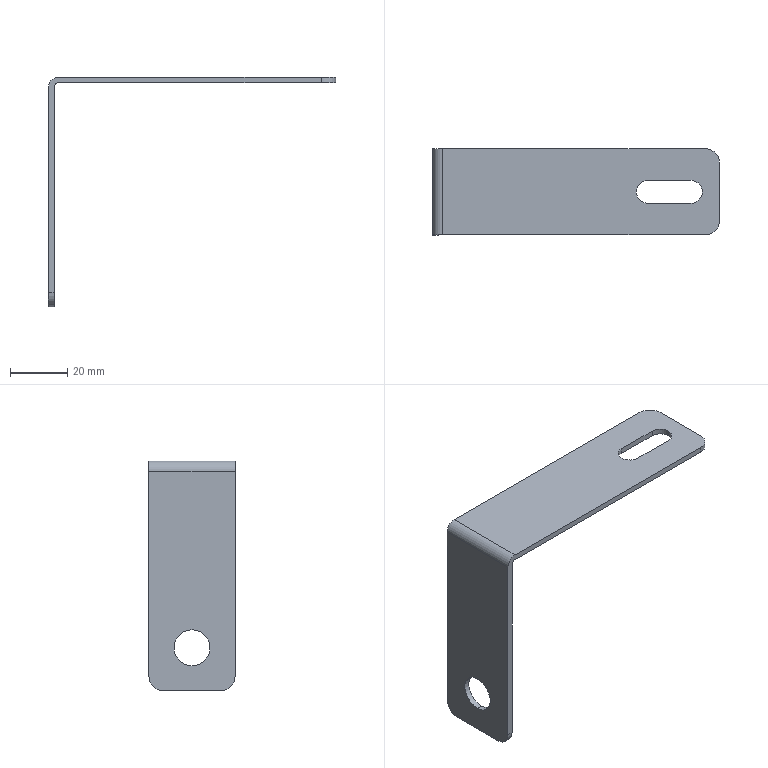Part | SolidWorks | features BaseBody 1 | 1 solid | 21 faces | box 100 x 30 x 80 mm | volume 9987 mm3 | cylinder 11 | plane 10 | commonest cylinder face diameters 10 x4 8 x3 12.5 x2 3 x1 7 x1
STEP:
#1=CARTESIAN_POINT('',(44.,0.,-2.));
#2=VERTEX_POINT('',#1);
#3=CARTESIAN_POINT('',(40.,4.,-2.));
#4=VERTEX_POINT('',#3);
#5=CARTESIAN_POINT('',(40.,0.,-2.));
#6=DIRECTION('',(0.,0.,1.));
#7=DIRECTION('',(1.,0.,0.));
#8=AXIS2_PLACEMENT_3D('',#5,#6,#7);
#9=CIRCLE('',#8,4.);
#10=EDGE_CURVE('',#2,#4,#9,.T.);
#11=ORIENTED_EDGE('',*,*,#10,.F.);
#12=CARTESIAN_POINT('',(44.,0.,0.));
#13=VERTEX_POINT('',#12);
#14=CARTESIAN_POINT('',(44.,0.,-10.));
#15=DIRECTION('',(0.,0.,1.));
#16=VECTOR('',#15,1000.);
#17=LINE('',#14,#16);
#18=EDGE_CURVE('',#2,#13,#17,.T.);
#19=ORIENTED_EDGE('',*,*,#18,.T.);
#20=CARTESIAN_POINT('',(40.,4.,0.));
#21=VERTEX_POINT('',#20);
#22=CARTESIAN_POINT('',(40.,0.,0.));
#23=DIRECTION('',(0.,0.,1.));
#24=DIRECTION('',(1.,0.,0.));
#25=AXIS2_PLACEMENT_3D('',#22,#23,#24);
#26=CIRCLE('',#25,4.);
#27=EDGE_CURVE('',#13,#21,#26,.T.);
#28=ORIENTED_EDGE('',*,*,#27,.T.);
#29=CARTESIAN_POINT('',(40.,4.,-10.));
#30=DIRECTION('',(0.,0.,-1.));
#31=VECTOR('',#30,1000.);
#32=LINE('',#29,#31);
#33=EDGE_CURVE('',#21,#4,#32,.T.);
#34=ORIENTED_EDGE('',*,*,#33,.T.);
#35=EDGE_LOOP('',(#11,#19,#28,#34));
#36=FACE_OUTER_BOUND('',#35,.T.);
#37=CARTESIAN_POINT('',(40.,0.,-10.));
#38=DIRECTION('',(0.,0.,1.));
#39=DIRECTION('',(1.,0.,0.));
#40=AXIS2_PLACEMENT_3D('',#37,#38,#39);
#41=CYLINDRICAL_SURFACE('',#40,4.);
#42=ADVANCED_FACE('',(#36),#41,.F.);
#43=CARTESIAN_POINT('',(-48.,0.,-71.25));
#44=VERTEX_POINT('',#43);
#45=CARTESIAN_POINT('',(-48.,0.,-58.75));
#46=VERTEX_POINT('',#45);
#47=CARTESIAN_POINT('',(-48.,0.,-65.));
#48=DIRECTION('',(-1.,0.,0.));
#49=DIRECTION('',(0.,0.,1.));
#50=AXIS2_PLACEMENT_3D('',#47,#48,#49);
#51=CIRCLE('',#50,6.25);
#52=EDGE_CURVE('',#44,#46,#51,.T.);
#53=ORIENTED_EDGE('',*,*,#52,.F.);
#54=CARTESIAN_POINT('',(-50.,0.,-71.25));
#55=VERTEX_POINT('',#54);
#56=CARTESIAN_POINT('',(-40.,0.,-71.25));
#57=DIRECTION('',(-1.,0.,0.));
#58=VECTOR('',#57,1000.);
#59=LINE('',#56,#58);
#60=EDGE_CURVE('',#44,#55,#59,.T.);
#61=ORIENTED_EDGE('',*,*,#60,.T.);
#62=CARTESIAN_POINT('',(-50.,0.,-58.75));
#63=VERTEX_POINT('',#62);
#64=CARTESIAN_POINT('',(-50.,0.,-65.));
#65=DIRECTION('',(1.,0.,0.));
#66=DIRECTION('',(0.,0.,1.));
#67=AXIS2_PLACEMENT_3D('',#64,#65,#66);
#68=CIRCLE('',#67,6.25);
#69=EDGE_CURVE('',#63,#55,#68,.T.);
#70=ORIENTED_EDGE('',*,*,#69,.F.);
#71=CARTESIAN_POINT('',(-40.,0.,-58.75));
#72=DIRECTION('',(-1.,0.,0.));
#73=VECTOR('',#72,1000.);
#74=LINE('',#71,#73);
#75=EDGE_CURVE('',#46,#63,#74,.T.);
#76=ORIENTED_EDGE('',*,*,#75,.F.);
#77=EDGE_LOOP('',(#53,#61,#70,#76));
#78=FACE_OUTER_BOUND('',#77,.T.);
#79=CARTESIAN_POINT('',(-40.,0.,-65.));
#80=DIRECTION('',(-1.,0.,0.));
#81=DIRECTION('',(0.,0.,1.));
#82=AXIS2_PLACEMENT_3D('',#79,#80,#81);
#83=CYLINDRICAL_SURFACE('',#82,6.25);
#84=ADVANCED_FACE('',(#78),#83,.F.);
#85=CARTESIAN_POINT('',(45.,15.,0.));
#86=VERTEX_POINT('',#85);
#87=CARTESIAN_POINT('',(50.,10.,0.));
#88=VERTEX_POINT('',#87);
#89=CARTESIAN_POINT('',(45.,10.,0.));
#90=DIRECTION('',(0.,0.,-1.));
#91=DIRECTION('',(1.,0.,0.));
#92=AXIS2_PLACEMENT_3D('',#89,#90,#91);
#93=CIRCLE('',#92,5.);
#94=EDGE_CURVE('',#86,#88,#93,.T.);
#95=ORIENTED_EDGE('',*,*,#94,.F.);
#96=CARTESIAN_POINT('',(-46.5,15.,0.));
#97=VERTEX_POINT('',#96);
#98=CARTESIAN_POINT('',(0.,15.,0.));
#99=DIRECTION('',(1.,0.,0.));
#100=VECTOR('',#99,1000.);
#101=LINE('',#98,#100);
#102=EDGE_CURVE('',#97,#86,#101,.T.);
#103=ORIENTED_EDGE('',*,*,#102,.F.);
#104=CARTESIAN_POINT('',(-46.5,-15.,0.));
#105=VERTEX_POINT('',#104);
#106=CARTESIAN_POINT('',(-46.5,0.,0.));
#107=DIRECTION('',(0.,1.,0.));
#108=VECTOR('',#107,1000.);
#109=LINE('',#106,#108);
#110=EDGE_CURVE('',#105,#97,#109,.T.);
#111=ORIENTED_EDGE('',*,*,#110,.F.);
#112=CARTESIAN_POINT('',(45.,-15.,0.));
#113=VERTEX_POINT('',#112);
#114=CARTESIAN_POINT('',(0.,-15.,0.));
#115=DIRECTION('',(-1.,0.,0.));
#116=VECTOR('',#115,1000.);
#117=LINE('',#114,#116);
#118=EDGE_CURVE('',#113,#105,#117,.T.);
#119=ORIENTED_EDGE('',*,*,#118,.F.);
#120=CARTESIAN_POINT('',(50.,-10.,0.));
#121=VERTEX_POINT('',#120);
#122=CARTESIAN_POINT('',(45.,-10.,0.));
#123=DIRECTION('',(0.,0.,-1.));
#124=DIRECTION('',(1.,0.,0.));
#125=AXIS2_PLACEMENT_3D('',#122,#123,#124);
#126=CIRCLE('',#125,5.);
#127=EDGE_CURVE('',#121,#113,#126,.T.);
#128=ORIENTED_EDGE('',*,*,#127,.F.);
#129=CARTESIAN_POINT('',(50.,0.,0.));
#130=DIRECTION('',(0.,-1.,0.));
#131=VECTOR('',#130,1000.);
#132=LINE('',#129,#131);
#133=EDGE_CURVE('',#88,#121,#132,.T.);
#134=ORIENTED_EDGE('',*,*,#133,.F.);
#135=EDGE_LOOP('',(#95,#103,#111,#119,#128,#134));
#136=FACE_OUTER_BOUND('',#135,.T.);
#137=CARTESIAN_POINT('',(25.,4.,0.));
#138=VERTEX_POINT('',#137);
#139=CARTESIAN_POINT('',(25.,-4.,0.));
#140=VERTEX_POINT('',#139);
#141=CARTESIAN_POINT('',(25.,0.,0.));
#142=DIRECTION('',(0.,0.,1.));
#143=DIRECTION('',(1.,0.,0.));
#144=AXIS2_PLACEMENT_3D('',#141,#142,#143);
#145=CIRCLE('',#144,4.);
#146=EDGE_CURVE('',#138,#140,#145,.T.);
#147=ORIENTED_EDGE('',*,*,#146,.F.);
#148=CARTESIAN_POINT('',(0.,4.,0.));
#149=DIRECTION('',(-1.,0.,0.));
#150=VECTOR('',#149,1000.);
#151=LINE('',#148,#150);
#152=EDGE_CURVE('',#21,#138,#151,.T.);
#153=ORIENTED_EDGE('',*,*,#152,.F.);
#154=ORIENTED_EDGE('',*,*,#27,.F.);
#155=CARTESIAN_POINT('',(40.,-4.,0.));
#156=VERTEX_POINT('',#155);
#157=CARTESIAN_POINT('',(40.,0.,0.));
#158=DIRECTION('',(0.,0.,1.));
#159=DIRECTION('',(1.,0.,0.));
#160=AXIS2_PLACEMENT_3D('',#157,#158,#159);
#161=CIRCLE('',#160,4.);
#162=EDGE_CURVE('',#156,#13,#161,.T.);
#163=ORIENTED_EDGE('',*,*,#162,.F.);
#164=CARTESIAN_POINT('',(0.,-4.,0.));
#165=DIRECTION('',(1.,0.,0.));
#166=VECTOR('',#165,1000.);
#167=LINE('',#164,#166);
#168=EDGE_CURVE('',#140,#156,#167,.T.);
#169=ORIENTED_EDGE('',*,*,#168,.F.);
#170=EDGE_LOOP('',(#147,#153,#154,#163,#169));
#171=FACE_BOUND('',#170,.T.);
#172=CARTESIAN_POINT('',(0.,0.,0.));
#173=DIRECTION('',(0.,0.,-1.));
#174=DIRECTION('',(-1.,0.,0.));
#175=AXIS2_PLACEMENT_3D('',#172,#173,#174);
#176=PLANE('',#175);
#177=ADVANCED_FACE('',(#136,#171),#176,.F.);
#178=ORIENTED_EDGE('',*,*,#133,.T.);
#179=CARTESIAN_POINT('',(50.,-10.,-2.));
#180=VERTEX_POINT('',#179);
#181=CARTESIAN_POINT('',(50.,-10.,-2.));
#182=DIRECTION('',(0.,0.,-1.));
#183=VECTOR('',#182,1000.);
#184=LINE('',#181,#183);
#185=EDGE_CURVE('',#121,#180,#184,.T.);
#186=ORIENTED_EDGE('',*,*,#185,.T.);
#187=CARTESIAN_POINT('',(50.,10.,-2.));
#188=VERTEX_POINT('',#187);
#189=CARTESIAN_POINT('',(50.,-15.,-2.));
#190=DIRECTION('',(0.,1.,0.));
#191=VECTOR('',#190,1000.);
#192=LINE('',#189,#191);
#193=EDGE_CURVE('',#180,#188,#192,.T.);
#194=ORIENTED_EDGE('',*,*,#193,.T.);
#195=CARTESIAN_POINT('',(50.,10.,-2.));
#196=DIRECTION('',(0.,0.,1.));
#197=VECTOR('',#196,1000.);
#198=LINE('',#195,#197);
#199=EDGE_CURVE('',#188,#88,#198,.T.);
#200=ORIENTED_EDGE('',*,*,#199,.T.);
#201=EDGE_LOOP('',(#178,#186,#194,#200));
#202=FACE_OUTER_BOUND('',#201,.T.);
#203=CARTESIAN_POINT('',(50.,-15.,-2.));
#204=DIRECTION('',(1.,0.,0.));
#205=DIRECTION('',(0.,0.,-1.));
#206=AXIS2_PLACEMENT_3D('',#203,#204,#205);
#207=PLANE('',#206);
#208=ADVANCED_FACE('',(#202),#207,.T.);
#209=ORIENTED_EDGE('',*,*,#94,.T.);
#210=ORIENTED_EDGE('',*,*,#199,.F.);
#211=CARTESIAN_POINT('',(45.,15.,-2.));
#212=VERTEX_POINT('',#211);
#213=CARTESIAN_POINT('',(45.,10.,-2.));
#214=DIRECTION('',(0.,0.,1.));
#215=DIRECTION('',(1.,0.,0.));
#216=AXIS2_PLACEMENT_3D('',#213,#214,#215);
#217=CIRCLE('',#216,5.);
#218=EDGE_CURVE('',#188,#212,#217,.T.);
#219=ORIENTED_EDGE('',*,*,#218,.T.);
#220=CARTESIAN_POINT('',(45.,15.,-2.));
#221=DIRECTION('',(0.,0.,1.));
#222=VECTOR('',#221,1000.);
#223=LINE('',#220,#222);
#224=EDGE_CURVE('',#212,#86,#223,.T.);
#225=ORIENTED_EDGE('',*,*,#224,.T.);
#226=EDGE_LOOP('',(#209,#210,#219,#225));
#227=FACE_OUTER_BOUND('',#226,.T.);
#228=CARTESIAN_POINT('',(45.,10.,-2.));
#229=DIRECTION('',(0.,0.,1.));
#230=DIRECTION('',(1.,0.,0.));
#231=AXIS2_PLACEMENT_3D('',#228,#229,#230);
#232=CYLINDRICAL_SURFACE('',#231,5.);
#233=ADVANCED_FACE('',(#227),#232,.T.);
#234=CARTESIAN_POINT('',(-46.5,15.,-2.));
#235=VERTEX_POINT('',#234);
#236=CARTESIAN_POINT('',(-50.,15.,-2.));
#237=DIRECTION('',(-1.,0.,0.));
#238=VECTOR('',#237,1000.);
#239=LINE('',#236,#238);
#240=EDGE_CURVE('',#212,#235,#239,.T.);
#241=ORIENTED_EDGE('',*,*,#240,.T.);
#242=CARTESIAN_POINT('',(-48.,15.,-3.5));
#243=VERTEX_POINT('',#242);
#244=CARTESIAN_POINT('',(-46.5,15.,-3.5));
#245=DIRECTION('',(0.,1.,0.));
#246=DIRECTION('',(0.,0.,1.));
#247=AXIS2_PLACEMENT_3D('',#244,#245,#246);
#248=CIRCLE('',#247,1.5);
#249=EDGE_CURVE('',#243,#235,#248,.T.);
#250=ORIENTED_EDGE('',*,*,#249,.F.);
#251=CARTESIAN_POINT('',(-48.,15.,-75.));
#252=VERTEX_POINT('',#251);
#253=CARTESIAN_POINT('',(-48.,15.,-2.));
#254=DIRECTION('',(0.,0.,-1.));
#255=VECTOR('',#254,1000.);
#256=LINE('',#253,#255);
#257=EDGE_CURVE('',#243,#252,#256,.T.);
#258=ORIENTED_EDGE('',*,*,#257,.T.);
#259=CARTESIAN_POINT('',(-50.,15.,-75.));
#260=VERTEX_POINT('',#259);
#261=CARTESIAN_POINT('',(-50.,15.,-75.));
#262=DIRECTION('',(-1.,0.,0.));
#263=VECTOR('',#262,1000.);
#264=LINE('',#261,#263);
#265=EDGE_CURVE('',#252,#260,#264,.T.);
#266=ORIENTED_EDGE('',*,*,#265,.T.);
#267=CARTESIAN_POINT('',(-50.,15.,-3.5));
#268=VERTEX_POINT('',#267);
#269=CARTESIAN_POINT('',(-50.,15.,0.));
#270=DIRECTION('',(0.,0.,-1.));
#271=VECTOR('',#270,1000.);
#272=LINE('',#269,#271);
#273=EDGE_CURVE('',#268,#260,#272,.T.);
#274=ORIENTED_EDGE('',*,*,#273,.F.);
#275=CARTESIAN_POINT('',(-46.5,15.,-3.5));
#276=DIRECTION('',(0.,-1.,0.));
#277=DIRECTION('',(0.,0.,1.));
#278=AXIS2_PLACEMENT_3D('',#275,#276,#277);
#279=CIRCLE('',#278,3.5);
#280=EDGE_CURVE('',#97,#268,#279,.T.);
#281=ORIENTED_EDGE('',*,*,#280,.F.);
#282=ORIENTED_EDGE('',*,*,#102,.T.);
#283=ORIENTED_EDGE('',*,*,#224,.F.);
#284=EDGE_LOOP('',(#241,#250,#258,#266,#274,#281,#282,#283));
#285=FACE_OUTER_BOUND('',#284,.T.);
#286=CARTESIAN_POINT('',(-50.,15.,-2.));
#287=DIRECTION('',(0.,1.,0.));
#288=DIRECTION('',(0.,0.,1.));
#289=AXIS2_PLACEMENT_3D('',#286,#287,#288);
#290=PLANE('',#289);
#291=ADVANCED_FACE('',(#285),#290,.T.);
#292=CARTESIAN_POINT('',(-50.,-15.,-3.5));
#293=VERTEX_POINT('',#292);
#294=CARTESIAN_POINT('',(-50.,15.,-3.5));
#295=DIRECTION('',(0.,-1.,0.));
#296=VECTOR('',#295,1000.);
#297=LINE('',#294,#296);
#298=EDGE_CURVE('',#268,#293,#297,.T.);
#299=ORIENTED_EDGE('',*,*,#298,.T.);
#300=CARTESIAN_POINT('',(-46.5,-15.,-3.5));
#301=DIRECTION('',(0.,1.,0.));
#302=DIRECTION('',(0.,0.,1.));
#303=AXIS2_PLACEMENT_3D('',#300,#301,#302);
#304=CIRCLE('',#303,3.5);
#305=EDGE_CURVE('',#293,#105,#304,.T.);
#306=ORIENTED_EDGE('',*,*,#305,.T.);
#307=ORIENTED_EDGE('',*,*,#110,.T.);
#308=ORIENTED_EDGE('',*,*,#280,.T.);
#309=EDGE_LOOP('',(#299,#306,#307,#308));
#310=FACE_OUTER_BOUND('',#309,.T.);
#311=CARTESIAN_POINT('',(-46.5,15.,-3.5));
#312=DIRECTION('',(0.,1.,0.));
#313=DIRECTION('',(0.,0.,1.));
#314=AXIS2_PLACEMENT_3D('',#311,#312,#313);
#315=CYLINDRICAL_SURFACE('',#314,3.5);
#316=ADVANCED_FACE('',(#310),#315,.T.);
#317=ORIENTED_EDGE('',*,*,#118,.T.);
#318=ORIENTED_EDGE('',*,*,#305,.F.);
#319=CARTESIAN_POINT('',(-50.,-15.,-75.));
#320=VERTEX_POINT('',#319);
#321=CARTESIAN_POINT('',(-50.,-15.,0.));
#322=DIRECTION('',(0.,0.,1.));
#323=VECTOR('',#322,1000.);
#324=LINE('',#321,#323);
#325=EDGE_CURVE('',#320,#293,#324,.T.);
#326=ORIENTED_EDGE('',*,*,#325,.F.);
#327=CARTESIAN_POINT('',(-48.,-15.,-75.));
#328=VERTEX_POINT('',#327);
#329=CARTESIAN_POINT('',(-50.,-15.,-75.));
#330=DIRECTION('',(1.,0.,0.));
#331=VECTOR('',#330,1000.);
#332=LINE('',#329,#331);
#333=EDGE_CURVE('',#320,#328,#332,.T.);
#334=ORIENTED_EDGE('',*,*,#333,.T.);
#335=CARTESIAN_POINT('',(-48.,-15.,-3.5));
#336=VERTEX_POINT('',#335);
#337=CARTESIAN_POINT('',(-48.,-15.,-80.));
#338=DIRECTION('',(0.,0.,1.));
#339=VECTOR('',#338,1000.);
#340=LINE('',#337,#339);
#341=EDGE_CURVE('',#328,#336,#340,.T.);
#342=ORIENTED_EDGE('',*,*,#341,.T.);
#343=CARTESIAN_POINT('',(-46.5,-15.,-2.));
#344=VERTEX_POINT('',#343);
#345=CARTESIAN_POINT('',(-46.5,-15.,-3.5));
#346=DIRECTION('',(0.,1.,0.));
#347=DIRECTION('',(0.,0.,1.));
#348=AXIS2_PLACEMENT_3D('',#345,#346,#347);
#349=CIRCLE('',#348,1.5);
#350=EDGE_CURVE('',#336,#344,#349,.T.);
#351=ORIENTED_EDGE('',*,*,#350,.T.);
#352=CARTESIAN_POINT('',(45.,-15.,-2.));
#353=VERTEX_POINT('',#352);
#354=CARTESIAN_POINT('',(-50.,-15.,-2.));
#355=DIRECTION('',(1.,0.,0.));
#356=VECTOR('',#355,1000.);
#357=LINE('',#354,#356);
#358=EDGE_CURVE('',#344,#353,#357,.T.);
#359=ORIENTED_EDGE('',*,*,#358,.T.);
#360=CARTESIAN_POINT('',(45.,-15.,-2.));
#361=DIRECTION('',(0.,0.,1.));
#362=VECTOR('',#361,1000.);
#363=LINE('',#360,#362);
#364=EDGE_CURVE('',#353,#113,#363,.T.);
#365=ORIENTED_EDGE('',*,*,#364,.T.);
#366=EDGE_LOOP('',(#317,#318,#326,#334,#342,#351,#359,#365));
#367=FACE_OUTER_BOUND('',#366,.T.);
#368=CARTESIAN_POINT('',(-50.,-15.,-2.));
#369=DIRECTION('',(0.,-1.,0.));
#370=DIRECTION('',(0.,0.,-1.));
#371=AXIS2_PLACEMENT_3D('',#368,#369,#370);
#372=PLANE('',#371);
#373=ADVANCED_FACE('',(#367),#372,.T.);
#374=ORIENTED_EDGE('',*,*,#127,.T.);
#375=ORIENTED_EDGE('',*,*,#364,.F.);
#376=CARTESIAN_POINT('',(45.,-10.,-2.));
#377=DIRECTION('',(0.,0.,1.));
#378=DIRECTION('',(1.,0.,0.));
#379=AXIS2_PLACEMENT_3D('',#376,#377,#378);
#380=CIRCLE('',#379,5.);
#381=EDGE_CURVE('',#353,#180,#380,.T.);
#382=ORIENTED_EDGE('',*,*,#381,.T.);
#383=ORIENTED_EDGE('',*,*,#185,.F.);
#384=EDGE_LOOP('',(#374,#375,#382,#383));
#385=FACE_OUTER_BOUND('',#384,.T.);
#386=CARTESIAN_POINT('',(45.,-10.,-2.));
#387=DIRECTION('',(0.,0.,1.));
#388=DIRECTION('',(1.,0.,0.));
#389=AXIS2_PLACEMENT_3D('',#386,#387,#388);
#390=CYLINDRICAL_SURFACE('',#389,5.);
#391=ADVANCED_FACE('',(#385),#390,.T.);
#392=CARTESIAN_POINT('',(25.,-4.,-2.));
#393=VERTEX_POINT('',#392);
#394=CARTESIAN_POINT('',(25.,-4.,-10.));
#395=DIRECTION('',(0.,0.,-1.));
#396=VECTOR('',#395,1000.);
#397=LINE('',#394,#396);
#398=EDGE_CURVE('',#140,#393,#397,.T.);
#399=ORIENTED_EDGE('',*,*,#398,.F.);
#400=ORIENTED_EDGE('',*,*,#168,.T.);
#401=CARTESIAN_POINT('',(40.,-4.,-2.));
#402=VERTEX_POINT('',#401);
#403=CARTESIAN_POINT('',(40.,-4.,-10.));
#404=DIRECTION('',(0.,0.,1.));
#405=VECTOR('',#404,1000.);
#406=LINE('',#403,#405);
#407=EDGE_CURVE('',#402,#156,#406,.T.);
#408=ORIENTED_EDGE('',*,*,#407,.F.);
#409=CARTESIAN_POINT('',(25.,-4.,-2.));
#410=DIRECTION('',(1.,0.,0.));
#411=VECTOR('',#410,1000.);
#412=LINE('',#409,#411);
#413=EDGE_CURVE('',#393,#402,#412,.T.);
#414=ORIENTED_EDGE('',*,*,#413,.F.);
#415=EDGE_LOOP('',(#399,#400,#408,#414));
#416=FACE_OUTER_BOUND('',#415,.T.);
#417=CARTESIAN_POINT('',(25.,-4.,-10.));
#418=DIRECTION('',(0.,-1.,0.));
#419=DIRECTION('',(0.,0.,-1.));
#420=AXIS2_PLACEMENT_3D('',#417,#418,#419);
#421=PLANE('',#420);
#422=ADVANCED_FACE('',(#416),#421,.F.);
#423=CARTESIAN_POINT('',(25.,4.,-2.));
#424=VERTEX_POINT('',#423);
#425=CARTESIAN_POINT('',(25.,4.,-10.));
#426=DIRECTION('',(0.,0.,-1.));
#427=VECTOR('',#426,1000.);
#428=LINE('',#425,#427);
#429=EDGE_CURVE('',#138,#424,#428,.T.);
#430=ORIENTED_EDGE('',*,*,#429,.F.);
#431=ORIENTED_EDGE('',*,*,#146,.T.);
#432=ORIENTED_EDGE('',*,*,#398,.T.);
#433=CARTESIAN_POINT('',(25.,0.,-2.));
#434=DIRECTION('',(0.,0.,1.));
#435=DIRECTION('',(1.,0.,0.));
#436=AXIS2_PLACEMENT_3D('',#433,#434,#435);
#437=CIRCLE('',#436,4.);
#438=EDGE_CURVE('',#424,#393,#437,.T.);
#439=ORIENTED_EDGE('',*,*,#438,.F.);
#440=EDGE_LOOP('',(#430,#431,#432,#439));
#441=FACE_OUTER_BOUND('',#440,.T.);
#442=CARTESIAN_POINT('',(25.,0.,-10.));
#443=DIRECTION('',(0.,0.,1.));
#444=DIRECTION('',(1.,0.,0.));
#445=AXIS2_PLACEMENT_3D('',#442,#443,#444);
#446=CYLINDRICAL_SURFACE('',#445,4.);
#447=ADVANCED_FACE('',(#441),#446,.F.);
#448=ORIENTED_EDGE('',*,*,#33,.F.);
#449=ORIENTED_EDGE('',*,*,#152,.T.);
#450=ORIENTED_EDGE('',*,*,#429,.T.);
#451=CARTESIAN_POINT('',(25.,4.,-2.));
#452=DIRECTION('',(-1.,0.,0.));
#453=VECTOR('',#452,1000.);
#454=LINE('',#451,#453);
#455=EDGE_CURVE('',#4,#424,#454,.T.);
#456=ORIENTED_EDGE('',*,*,#455,.F.);
#457=EDGE_LOOP('',(#448,#449,#450,#456));
#458=FACE_OUTER_BOUND('',#457,.T.);
#459=CARTESIAN_POINT('',(25.,4.,-10.));
#460=DIRECTION('',(0.,1.,0.));
#461=DIRECTION('',(-1.,0.,0.));
#462=AXIS2_PLACEMENT_3D('',#459,#460,#461);
#463=PLANE('',#462);
#464=ADVANCED_FACE('',(#458),#463,.F.);
#465=ORIENTED_EDGE('',*,*,#18,.F.);
#466=CARTESIAN_POINT('',(40.,0.,-2.));
#467=DIRECTION('',(0.,0.,1.));
#468=DIRECTION('',(1.,0.,0.));
#469=AXIS2_PLACEMENT_3D('',#466,#467,#468);
#470=CIRCLE('',#469,4.);
#471=EDGE_CURVE('',#402,#2,#470,.T.);
#472=ORIENTED_EDGE('',*,*,#471,.F.);
#473=ORIENTED_EDGE('',*,*,#407,.T.);
#474=ORIENTED_EDGE('',*,*,#162,.T.);
#475=EDGE_LOOP('',(#465,#472,#473,#474));
#476=FACE_OUTER_BOUND('',#475,.T.);
#477=CARTESIAN_POINT('',(40.,0.,-10.));
#478=DIRECTION('',(0.,0.,1.));
#479=DIRECTION('',(1.,0.,0.));
#480=AXIS2_PLACEMENT_3D('',#477,#478,#479);
#481=CYLINDRICAL_SURFACE('',#480,4.);
#482=ADVANCED_FACE('',(#476),#481,.F.);
#483=ORIENTED_EDGE('',*,*,#358,.F.);
#484=CARTESIAN_POINT('',(-46.5,0.,-2.));
#485=DIRECTION('',(0.,1.,0.));
#486=VECTOR('',#485,1000.);
#487=LINE('',#484,#486);
#488=EDGE_CURVE('',#344,#235,#487,.T.);
#489=ORIENTED_EDGE('',*,*,#488,.T.);
#490=ORIENTED_EDGE('',*,*,#240,.F.);
#491=ORIENTED_EDGE('',*,*,#218,.F.);
#492=ORIENTED_EDGE('',*,*,#193,.F.);
#493=ORIENTED_EDGE('',*,*,#381,.F.);
#494=EDGE_LOOP('',(#483,#489,#490,#491,#492,#493));
#495=FACE_OUTER_BOUND('',#494,.T.);
#496=ORIENTED_EDGE('',*,*,#471,.T.);
#497=ORIENTED_EDGE('',*,*,#10,.T.);
#498=ORIENTED_EDGE('',*,*,#455,.T.);
#499=ORIENTED_EDGE('',*,*,#438,.T.);
#500=ORIENTED_EDGE('',*,*,#413,.T.);
#501=EDGE_LOOP('',(#496,#497,#498,#499,#500));
#502=FACE_BOUND('',#501,.T.);
#503=CARTESIAN_POINT('',(0.,0.,-2.));
#504=DIRECTION('',(0.,0.,-1.));
#505=DIRECTION('',(-1.,0.,0.));
#506=AXIS2_PLACEMENT_3D('',#503,#504,#505);
#507=PLANE('',#506);
#508=ADVANCED_FACE('',(#495,#502),#507,.T.);
#509=ORIENTED_EDGE('',*,*,#325,.T.);
#510=ORIENTED_EDGE('',*,*,#298,.F.);
#511=ORIENTED_EDGE('',*,*,#273,.T.);
#512=CARTESIAN_POINT('',(-50.,10.,-80.));
#513=VERTEX_POINT('',#512);
#514=CARTESIAN_POINT('',(-50.,10.,-75.));
#515=DIRECTION('',(-1.,0.,0.));
#516=DIRECTION('',(0.,0.,-1.));
#517=AXIS2_PLACEMENT_3D('',#514,#515,#516);
#518=CIRCLE('',#517,5.);
#519=EDGE_CURVE('',#260,#513,#518,.T.);
#520=ORIENTED_EDGE('',*,*,#519,.T.);
#521=CARTESIAN_POINT('',(-50.,-10.,-80.));
#522=VERTEX_POINT('',#521);
#523=CARTESIAN_POINT('',(-50.,0.,-80.));
#524=DIRECTION('',(0.,-1.,0.));
#525=VECTOR('',#524,1000.);
#526=LINE('',#523,#525);
#527=EDGE_CURVE('',#513,#522,#526,.T.);
#528=ORIENTED_EDGE('',*,*,#527,.T.);
#529=CARTESIAN_POINT('',(-50.,-10.,-75.));
#530=DIRECTION('',(-1.,0.,0.));
#531=DIRECTION('',(0.,0.,-1.));
#532=AXIS2_PLACEMENT_3D('',#529,#530,#531);
#533=CIRCLE('',#532,5.);
#534=EDGE_CURVE('',#522,#320,#533,.T.);
#535=ORIENTED_EDGE('',*,*,#534,.T.);
#536=EDGE_LOOP('',(#509,#510,#511,#520,#528,#535));
#537=FACE_OUTER_BOUND('',#536,.T.);
#538=ORIENTED_EDGE('',*,*,#69,.T.);
#539=CARTESIAN_POINT('',(-50.,0.,-65.));
#540=DIRECTION('',(1.,0.,0.));
#541=DIRECTION('',(0.,0.,1.));
#542=AXIS2_PLACEMENT_3D('',#539,#540,#541);
#543=CIRCLE('',#542,6.25);
#544=EDGE_CURVE('',#55,#63,#543,.T.);
#545=ORIENTED_EDGE('',*,*,#544,.T.);
#546=EDGE_LOOP('',(#538,#545));
#547=FACE_BOUND('',#546,.T.);
#548=CARTESIAN_POINT('',(-50.,0.,0.));
#549=DIRECTION('',(-1.,0.,0.));
#550=DIRECTION('',(0.,0.,1.));
#551=AXIS2_PLACEMENT_3D('',#548,#549,#550);
#552=PLANE('',#551);
#553=ADVANCED_FACE('',(#537,#547),#552,.T.);
#554=ORIENTED_EDGE('',*,*,#350,.F.);
#555=CARTESIAN_POINT('',(-48.,15.,-3.5));
#556=DIRECTION('',(0.,-1.,0.));
#557=VECTOR('',#556,1000.);
#558=LINE('',#555,#557);
#559=EDGE_CURVE('',#243,#336,#558,.T.);
#560=ORIENTED_EDGE('',*,*,#559,.F.);
#561=ORIENTED_EDGE('',*,*,#249,.T.);
#562=ORIENTED_EDGE('',*,*,#488,.F.);
#563=EDGE_LOOP('',(#554,#560,#561,#562));
#564=FACE_OUTER_BOUND('',#563,.T.);
#565=CARTESIAN_POINT('',(-46.5,15.,-3.5));
#566=DIRECTION('',(0.,1.,0.));
#567=DIRECTION('',(0.,0.,1.));
#568=AXIS2_PLACEMENT_3D('',#565,#566,#567);
#569=CYLINDRICAL_SURFACE('',#568,1.5);
#570=ADVANCED_FACE('',(#564),#569,.F.);
#571=CARTESIAN_POINT('',(-48.,-10.,-80.));
#572=VERTEX_POINT('',#571);
#573=CARTESIAN_POINT('',(-48.,-10.,-75.));
#574=DIRECTION('',(-1.,0.,0.));
#575=DIRECTION('',(0.,0.,-1.));
#576=AXIS2_PLACEMENT_3D('',#573,#574,#575);
#577=CIRCLE('',#576,5.);
#578=EDGE_CURVE('',#572,#328,#577,.T.);
#579=ORIENTED_EDGE('',*,*,#578,.T.);
#580=ORIENTED_EDGE('',*,*,#333,.F.);
#581=ORIENTED_EDGE('',*,*,#534,.F.);
#582=CARTESIAN_POINT('',(-50.,-10.,-80.));
#583=DIRECTION('',(1.,0.,0.));
#584=VECTOR('',#583,1000.);
#585=LINE('',#582,#584);
#586=EDGE_CURVE('',#522,#572,#585,.T.);
#587=ORIENTED_EDGE('',*,*,#586,.T.);
#588=EDGE_LOOP('',(#579,#580,#581,#587));
#589=FACE_OUTER_BOUND('',#588,.T.);
#590=CARTESIAN_POINT('',(-50.,-10.,-75.));
#591=DIRECTION('',(1.,0.,0.));
#592=DIRECTION('',(0.,0.,-1.));
#593=AXIS2_PLACEMENT_3D('',#590,#591,#592);
#594=CYLINDRICAL_SURFACE('',#593,5.);
#595=ADVANCED_FACE('',(#589),#594,.T.);
#596=CARTESIAN_POINT('',(-48.,10.,-80.));
#597=VERTEX_POINT('',#596);
#598=CARTESIAN_POINT('',(-48.,15.,-80.));
#599=DIRECTION('',(0.,-1.,0.));
#600=VECTOR('',#599,1000.);
#601=LINE('',#598,#600);
#602=EDGE_CURVE('',#597,#572,#601,.T.);
#603=ORIENTED_EDGE('',*,*,#602,.T.);
#604=ORIENTED_EDGE('',*,*,#586,.F.);
#605=ORIENTED_EDGE('',*,*,#527,.F.);
#606=CARTESIAN_POINT('',(-50.,10.,-80.));
#607=DIRECTION('',(1.,0.,0.));
#608=VECTOR('',#607,1000.);
#609=LINE('',#606,#608);
#610=EDGE_CURVE('',#513,#597,#609,.T.);
#611=ORIENTED_EDGE('',*,*,#610,.T.);
#612=EDGE_LOOP('',(#603,#604,#605,#611));
#613=FACE_OUTER_BOUND('',#612,.T.);
#614=CARTESIAN_POINT('',(-50.,15.,-80.));
#615=DIRECTION('',(0.,0.,-1.));
#616=DIRECTION('',(-1.,0.,0.));
#617=AXIS2_PLACEMENT_3D('',#614,#615,#616);
#618=PLANE('',#617);
#619=ADVANCED_FACE('',(#613),#618,.T.);
#620=CARTESIAN_POINT('',(-48.,10.,-75.));
#621=DIRECTION('',(-1.,0.,0.));
#622=DIRECTION('',(0.,0.,-1.));
#623=AXIS2_PLACEMENT_3D('',#620,#621,#622);
#624=CIRCLE('',#623,5.);
#625=EDGE_CURVE('',#252,#597,#624,.T.);
#626=ORIENTED_EDGE('',*,*,#625,.T.);
#627=ORIENTED_EDGE('',*,*,#610,.F.);
#628=ORIENTED_EDGE('',*,*,#519,.F.);
#629=ORIENTED_EDGE('',*,*,#265,.F.);
#630=EDGE_LOOP('',(#626,#627,#628,#629));
#631=FACE_OUTER_BOUND('',#630,.T.);
#632=CARTESIAN_POINT('',(-50.,10.,-75.));
#633=DIRECTION('',(1.,0.,0.));
#634=DIRECTION('',(0.,0.,-1.));
#635=AXIS2_PLACEMENT_3D('',#632,#633,#634);
#636=CYLINDRICAL_SURFACE('',#635,5.);
#637=ADVANCED_FACE('',(#631),#636,.T.);
#638=ORIENTED_EDGE('',*,*,#60,.F.);
#639=CARTESIAN_POINT('',(-48.,0.,-65.));
#640=DIRECTION('',(-1.,0.,0.));
#641=DIRECTION('',(0.,0.,1.));
#642=AXIS2_PLACEMENT_3D('',#639,#640,#641);
#643=CIRCLE('',#642,6.25);
#644=EDGE_CURVE('',#46,#44,#643,.T.);
#645=ORIENTED_EDGE('',*,*,#644,.F.);
#646=ORIENTED_EDGE('',*,*,#75,.T.);
#647=ORIENTED_EDGE('',*,*,#544,.F.);
#648=EDGE_LOOP('',(#638,#645,#646,#647));
#649=FACE_OUTER_BOUND('',#648,.T.);
#650=CARTESIAN_POINT('',(-40.,0.,-65.));
#651=DIRECTION('',(-1.,0.,0.));
#652=DIRECTION('',(0.,0.,1.));
#653=AXIS2_PLACEMENT_3D('',#650,#651,#652);
#654=CYLINDRICAL_SURFACE('',#653,6.25);
#655=ADVANCED_FACE('',(#649),#654,.F.);
#656=ORIENTED_EDGE('',*,*,#625,.F.);
#657=ORIENTED_EDGE('',*,*,#257,.F.);
#658=ORIENTED_EDGE('',*,*,#559,.T.);
#659=ORIENTED_EDGE('',*,*,#341,.F.);
#660=ORIENTED_EDGE('',*,*,#578,.F.);
#661=ORIENTED_EDGE('',*,*,#602,.F.);
#662=EDGE_LOOP('',(#656,#657,#658,#659,#660,#661));
#663=FACE_OUTER_BOUND('',#662,.T.);
#664=ORIENTED_EDGE('',*,*,#644,.T.);
#665=ORIENTED_EDGE('',*,*,#52,.T.);
#666=EDGE_LOOP('',(#664,#665));
#667=FACE_BOUND('',#666,.T.);
#668=CARTESIAN_POINT('',(-48.,0.,0.));
#669=DIRECTION('',(-1.,0.,0.));
#670=DIRECTION('',(0.,0.,1.));
#671=AXIS2_PLACEMENT_3D('',#668,#669,#670);
#672=PLANE('',#671);
#673=ADVANCED_FACE('',(#663,#667),#672,.F.);
#674=CLOSED_SHELL('',(#42,#84,#177,#208,#233,#291,#316,#373,#391,#422,#447,#464,#482,#508,#553,#570,#595,#619,#637,#655,#673));
#675=MANIFOLD_SOLID_BREP('',#674);
#676=CARTESIAN_POINT('',(0.,0.,0.));
#677=DIRECTION('',(0.,0.,1.));
#678=DIRECTION('',(1.,0.,0.));
#679=AXIS2_PLACEMENT_3D('',#676,#677,#678);
#680=(LENGTH_UNIT()NAMED_UNIT(*)SI_UNIT(.MILLI.,.METRE.));
#681=UNCERTAINTY_MEASURE_WITH_UNIT(LENGTH_MEASURE(0.00001),#680,'','');
#682=(NAMED_UNIT(*)PLANE_ANGLE_UNIT()SI_UNIT($,.RADIAN.));
#683=(NAMED_UNIT(*)SI_UNIT($,.STERADIAN.)SOLID_ANGLE_UNIT());
#684=(GEOMETRIC_REPRESENTATION_CONTEXT(3)GLOBAL_UNCERTAINTY_ASSIGNED_CONTEXT((#681))GLOBAL_UNIT_ASSIGNED_CONTEXT((#680,#682,#683))REPRESENTATION_CONTEXT('',''));
#685=ADVANCED_BREP_SHAPE_REPRESENTATION('',(#675,#679),#684);